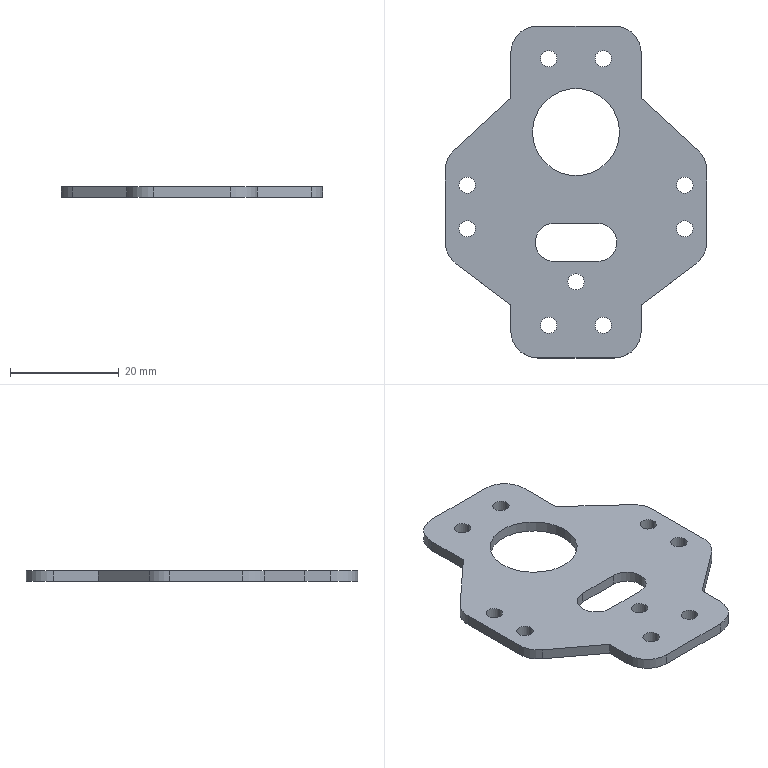Part | STEP file | Gripper (new)_1 | 1 solid | 47 faces | box 48 x 61 x 2 mm | volume 3505 mm3 | cylinder 31 | plane 16 | commonest cylinder face diameters 3 x18 10 x8 7 x3 16 x2